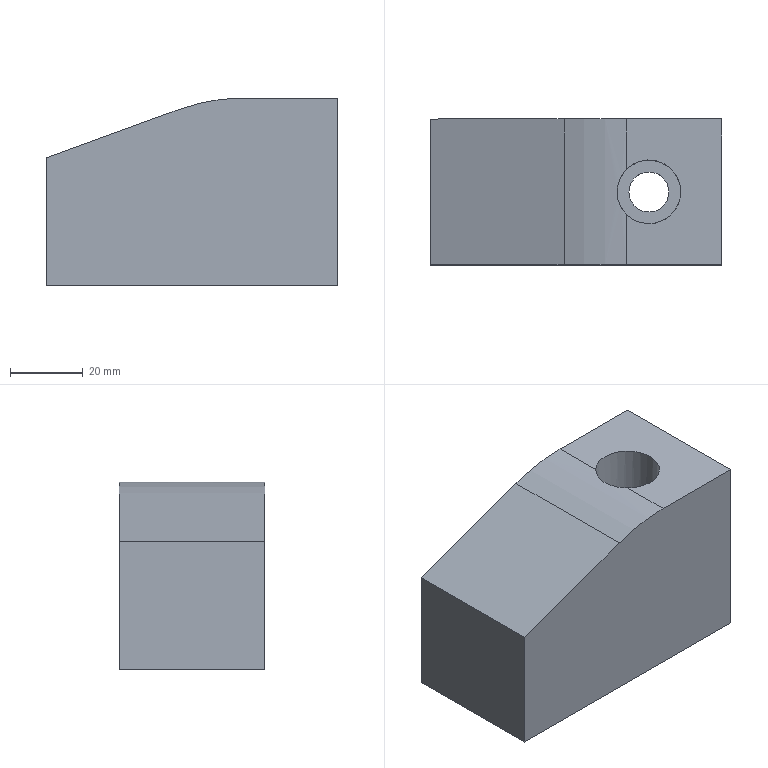Part | NX | features MAIN_BODY 2 | 1 solid | 11 faces | box 80 x 40 x 51.5 mm | volume 139981 mm3 | plane 8 | cylinder 3 | commonest cylinder face diameters 11 x1 17.5 x1 100 x1
STEP:
#1=CARTESIAN_POINT('',(-1566.191,130.,-4.));
#2=VERTEX_POINT('',#1);
#3=CARTESIAN_POINT('',(-1540.,130.,-4.));
#4=VERTEX_POINT('',#3);
#5=CARTESIAN_POINT('',(-1625.,130.,-4.));
#6=DIRECTION('',(-1.,0.,0.));
#7=VECTOR('',#6,1000.);
#8=LINE('',#5,#7);
#9=EDGE_CURVE('',#2,#4,#8,.F.);
#10=ORIENTED_EDGE('',*,*,#9,.F.);
#11=CARTESIAN_POINT('',(-1583.278,130.,-7.01));
#12=VERTEX_POINT('',#11);
#13=CARTESIAN_POINT('',(-1566.191,130.,-54.));
#14=DIRECTION('',(0.,1.,0.));
#15=DIRECTION('',(0.,0.,1.));
#16=AXIS2_PLACEMENT_3D('',#13,#14,#15);
#17=CIRCLE('',#16,50.);
#18=EDGE_CURVE('',#2,#12,#17,.F.);
#19=ORIENTED_EDGE('',*,*,#18,.T.);
#20=CARTESIAN_POINT('',(-1620.,130.,-20.364));
#21=VERTEX_POINT('',#20);
#22=CARTESIAN_POINT('',(-1619.161,130.,-20.058));
#23=DIRECTION('',(-0.9398,0.,-0.3417));
#24=VECTOR('',#23,1000.);
#25=LINE('',#22,#24);
#26=EDGE_CURVE('',#12,#21,#25,.T.);
#27=ORIENTED_EDGE('',*,*,#26,.T.);
#28=CARTESIAN_POINT('',(-1620.,130.,-55.5));
#29=VERTEX_POINT('',#28);
#30=CARTESIAN_POINT('',(-1620.,130.,-4.));
#31=DIRECTION('',(0.,0.,1.));
#32=VECTOR('',#31,1000.);
#33=LINE('',#30,#32);
#34=EDGE_CURVE('',#21,#29,#33,.F.);
#35=ORIENTED_EDGE('',*,*,#34,.T.);
#36=CARTESIAN_POINT('',(-1540.,130.,-55.5));
#37=VERTEX_POINT('',#36);
#38=CARTESIAN_POINT('',(-1625.,130.,-55.5));
#39=DIRECTION('',(-1.,0.,0.));
#40=VECTOR('',#39,1000.);
#41=LINE('',#38,#40);
#42=EDGE_CURVE('',#29,#37,#41,.F.);
#43=ORIENTED_EDGE('',*,*,#42,.T.);
#44=CARTESIAN_POINT('',(-1540.,130.,-4.));
#45=DIRECTION('',(0.,0.,1.));
#46=VECTOR('',#45,1000.);
#47=LINE('',#44,#46);
#48=EDGE_CURVE('',#4,#37,#47,.F.);
#49=ORIENTED_EDGE('',*,*,#48,.F.);
#50=EDGE_LOOP('',(#10,#19,#27,#35,#43,#49));
#51=FACE_BOUND('',#50,.T.);
#52=CARTESIAN_POINT('',(-1625.,130.,-4.));
#53=DIRECTION('',(0.,1.,0.));
#54=DIRECTION('',(0.,0.,-1.));
#55=AXIS2_PLACEMENT_3D('',#52,#53,#54);
#56=PLANE('',#55);
#57=ADVANCED_FACE('',(#51),#56,.F.);
#58=CARTESIAN_POINT('',(-1620.,170.,-20.364));
#59=VERTEX_POINT('',#58);
#60=CARTESIAN_POINT('',(-1583.278,170.,-7.01));
#61=VERTEX_POINT('',#60);
#62=CARTESIAN_POINT('',(-1619.161,170.,-20.058));
#63=DIRECTION('',(-0.9398,0.,-0.3417));
#64=VECTOR('',#63,1000.);
#65=LINE('',#62,#64);
#66=EDGE_CURVE('',#59,#61,#65,.F.);
#67=ORIENTED_EDGE('',*,*,#66,.T.);
#68=CARTESIAN_POINT('',(-1566.191,170.,-4.));
#69=VERTEX_POINT('',#68);
#70=CARTESIAN_POINT('',(-1566.191,170.,-54.));
#71=DIRECTION('',(0.,1.,0.));
#72=DIRECTION('',(0.,0.,1.));
#73=AXIS2_PLACEMENT_3D('',#70,#71,#72);
#74=CIRCLE('',#73,50.);
#75=EDGE_CURVE('',#61,#69,#74,.T.);
#76=ORIENTED_EDGE('',*,*,#75,.T.);
#77=CARTESIAN_POINT('',(-1540.,170.,-4.));
#78=VERTEX_POINT('',#77);
#79=CARTESIAN_POINT('',(-1625.,170.,-4.));
#80=DIRECTION('',(1.,0.,0.));
#81=VECTOR('',#80,1000.);
#82=LINE('',#79,#81);
#83=EDGE_CURVE('',#69,#78,#82,.T.);
#84=ORIENTED_EDGE('',*,*,#83,.T.);
#85=CARTESIAN_POINT('',(-1540.,170.,-55.5));
#86=VERTEX_POINT('',#85);
#87=CARTESIAN_POINT('',(-1540.,170.,-4.));
#88=DIRECTION('',(0.,0.,-1.));
#89=VECTOR('',#88,1000.);
#90=LINE('',#87,#89);
#91=EDGE_CURVE('',#78,#86,#90,.T.);
#92=ORIENTED_EDGE('',*,*,#91,.T.);
#93=CARTESIAN_POINT('',(-1620.,170.,-55.5));
#94=VERTEX_POINT('',#93);
#95=CARTESIAN_POINT('',(-1625.,170.,-55.5));
#96=DIRECTION('',(-1.,0.,0.));
#97=VECTOR('',#96,1000.);
#98=LINE('',#95,#97);
#99=EDGE_CURVE('',#86,#94,#98,.T.);
#100=ORIENTED_EDGE('',*,*,#99,.T.);
#101=CARTESIAN_POINT('',(-1620.,170.,-4.));
#102=DIRECTION('',(0.,0.,-1.));
#103=VECTOR('',#102,1000.);
#104=LINE('',#101,#103);
#105=EDGE_CURVE('',#59,#94,#104,.T.);
#106=ORIENTED_EDGE('',*,*,#105,.F.);
#107=EDGE_LOOP('',(#67,#76,#84,#92,#100,#106));
#108=FACE_BOUND('',#107,.T.);
#109=CARTESIAN_POINT('',(-1625.,170.,-4.));
#110=DIRECTION('',(0.,1.,0.));
#111=DIRECTION('',(0.,0.,-1.));
#112=AXIS2_PLACEMENT_3D('',#109,#110,#111);
#113=PLANE('',#112);
#114=ADVANCED_FACE('',(#108),#113,.T.);
#115=ORIENTED_EDGE('',*,*,#48,.T.);
#116=CARTESIAN_POINT('',(-1540.,135.,-55.5));
#117=DIRECTION('',(0.,-1.,0.));
#118=VECTOR('',#117,1000.);
#119=LINE('',#116,#118);
#120=EDGE_CURVE('',#86,#37,#119,.T.);
#121=ORIENTED_EDGE('',*,*,#120,.F.);
#122=ORIENTED_EDGE('',*,*,#91,.F.);
#123=CARTESIAN_POINT('',(-1540.,135.,-4.));
#124=DIRECTION('',(0.,1.,0.));
#125=VECTOR('',#124,1000.);
#126=LINE('',#123,#125);
#127=EDGE_CURVE('',#4,#78,#126,.T.);
#128=ORIENTED_EDGE('',*,*,#127,.F.);
#129=EDGE_LOOP('',(#115,#121,#122,#128));
#130=FACE_BOUND('',#129,.T.);
#131=CARTESIAN_POINT('',(-1540.,135.,-4.));
#132=DIRECTION('',(-1.,0.,0.));
#133=DIRECTION('',(0.,0.,1.));
#134=AXIS2_PLACEMENT_3D('',#131,#132,#133);
#135=PLANE('',#134);
#136=ADVANCED_FACE('',(#130),#135,.F.);
#137=ORIENTED_EDGE('',*,*,#105,.T.);
#138=CARTESIAN_POINT('',(-1620.,135.,-55.5));
#139=DIRECTION('',(0.,-1.,0.));
#140=VECTOR('',#139,1000.);
#141=LINE('',#138,#140);
#142=EDGE_CURVE('',#94,#29,#141,.T.);
#143=ORIENTED_EDGE('',*,*,#142,.T.);
#144=ORIENTED_EDGE('',*,*,#34,.F.);
#145=CARTESIAN_POINT('',(-1620.,135.,-20.364));
#146=DIRECTION('',(0.,-1.,0.));
#147=VECTOR('',#146,1000.);
#148=LINE('',#145,#147);
#149=EDGE_CURVE('',#21,#59,#148,.F.);
#150=ORIENTED_EDGE('',*,*,#149,.T.);
#151=EDGE_LOOP('',(#137,#143,#144,#150));
#152=FACE_BOUND('',#151,.T.);
#153=CARTESIAN_POINT('',(-1620.,135.,-4.));
#154=DIRECTION('',(-1.,0.,0.));
#155=DIRECTION('',(0.,0.,1.));
#156=AXIS2_PLACEMENT_3D('',#153,#154,#155);
#157=PLANE('',#156);
#158=ADVANCED_FACE('',(#152),#157,.T.);
#159=CARTESIAN_POINT('',(-1566.191,156.183,-4.));
#160=VERTEX_POINT('',#159);
#161=CARTESIAN_POINT('',(-1566.191,135.,-4.));
#162=DIRECTION('',(0.,1.,0.));
#163=VECTOR('',#162,1000.);
#164=LINE('',#161,#163);
#165=EDGE_CURVE('',#69,#160,#164,.F.);
#166=ORIENTED_EDGE('',*,*,#165,.T.);
#167=CARTESIAN_POINT('',(-1566.191,143.817,-4.));
#168=VERTEX_POINT('',#167);
#169=CARTESIAN_POINT('',(-1560.,150.,-4.));
#170=DIRECTION('',(0.,0.,-1.));
#171=DIRECTION('',(1.,0.,0.));
#172=AXIS2_PLACEMENT_3D('',#169,#170,#171);
#173=CIRCLE('',#172,8.75);
#174=EDGE_CURVE('',#168,#160,#173,.F.);
#175=ORIENTED_EDGE('',*,*,#174,.F.);
#176=CARTESIAN_POINT('',(-1566.191,135.,-4.));
#177=DIRECTION('',(0.,1.,0.));
#178=VECTOR('',#177,1000.);
#179=LINE('',#176,#178);
#180=EDGE_CURVE('',#168,#2,#179,.F.);
#181=ORIENTED_EDGE('',*,*,#180,.T.);
#182=ORIENTED_EDGE('',*,*,#9,.T.);
#183=ORIENTED_EDGE('',*,*,#127,.T.);
#184=ORIENTED_EDGE('',*,*,#83,.F.);
#185=EDGE_LOOP('',(#166,#175,#181,#182,#183,#184));
#186=FACE_BOUND('',#185,.T.);
#187=CARTESIAN_POINT('',(-1625.,135.,-4.));
#188=DIRECTION('',(0.,0.,1.));
#189=DIRECTION('',(0.,1.,0.));
#190=AXIS2_PLACEMENT_3D('',#187,#188,#189);
#191=PLANE('',#190);
#192=ADVANCED_FACE('',(#186),#191,.T.);
#193=ORIENTED_EDGE('',*,*,#26,.F.);
#194=CARTESIAN_POINT('',(-1583.278,135.,-7.01));
#195=DIRECTION('',(0.,-1.,0.));
#196=VECTOR('',#195,1000.);
#197=LINE('',#194,#196);
#198=EDGE_CURVE('',#12,#61,#197,.F.);
#199=ORIENTED_EDGE('',*,*,#198,.T.);
#200=ORIENTED_EDGE('',*,*,#66,.F.);
#201=ORIENTED_EDGE('',*,*,#149,.F.);
#202=EDGE_LOOP('',(#193,#199,#200,#201));
#203=FACE_BOUND('',#202,.T.);
#204=CARTESIAN_POINT('',(-1630.,135.,-24.));
#205=DIRECTION('',(0.3417,0.,-0.9398));
#206=DIRECTION('',(-0.9398,0.,-0.3417));
#207=AXIS2_PLACEMENT_3D('',#204,#205,#206);
#208=PLANE('',#207);
#209=ADVANCED_FACE('',(#203),#208,.F.);
#210=ORIENTED_EDGE('',*,*,#180,.F.);
#211=CARTESIAN_POINT('',(-1566.191,156.183,-4.));
#212=CARTESIAN_POINT('',(-1567.825,154.548,-4.));
#213=CARTESIAN_POINT('',(-1569.686,150.004,-4.131));
#214=CARTESIAN_POINT('',(-1567.803,145.431,-4.));
#215=CARTESIAN_POINT('',(-1566.191,143.817,-4.));
#216=B_SPLINE_CURVE_WITH_KNOTS('',3,(#211,#212,#213,#214,#215),.UNSPECIFIED.,.F.,.F.,(4,1,4),(0.002912,0.009748,0.01658),.UNSPECIFIED.);
#217=EDGE_CURVE('',#168,#160,#216,.F.);
#218=ORIENTED_EDGE('',*,*,#217,.T.);
#219=ORIENTED_EDGE('',*,*,#165,.F.);
#220=ORIENTED_EDGE('',*,*,#75,.F.);
#221=ORIENTED_EDGE('',*,*,#198,.F.);
#222=ORIENTED_EDGE('',*,*,#18,.F.);
#223=EDGE_LOOP('',(#210,#218,#219,#220,#221,#222));
#224=FACE_BOUND('',#223,.T.);
#225=CARTESIAN_POINT('',(-1566.191,135.,-54.));
#226=DIRECTION('',(0.,1.,0.));
#227=DIRECTION('',(0.,0.,1.));
#228=AXIS2_PLACEMENT_3D('',#225,#226,#227);
#229=CYLINDRICAL_SURFACE('',#228,50.);
#230=ADVANCED_FACE('',(#224),#229,.T.);
#231=CARTESIAN_POINT('',(-1565.5,150.,-38.5));
#232=VERTEX_POINT('',#231);
#233=CARTESIAN_POINT('',(-1560.,150.,-38.5));
#234=DIRECTION('',(0.,0.,-1.));
#235=DIRECTION('',(-1.,0.,0.));
#236=AXIS2_PLACEMENT_3D('',#233,#234,#235);
#237=CIRCLE('',#236,5.5);
#238=EDGE_CURVE('',#232,#232,#237,.T.);
#239=ORIENTED_EDGE('',*,*,#238,.F.);
#240=EDGE_LOOP('',(#239));
#241=FACE_BOUND('',#240,.T.);
#242=CARTESIAN_POINT('',(-1565.5,150.,-55.5));
#243=VERTEX_POINT('',#242);
#244=CARTESIAN_POINT('',(-1560.,150.,-55.5));
#245=DIRECTION('',(0.,0.,-1.));
#246=DIRECTION('',(-1.,0.,0.));
#247=AXIS2_PLACEMENT_3D('',#244,#245,#246);
#248=CIRCLE('',#247,5.5);
#249=EDGE_CURVE('',#243,#243,#248,.T.);
#250=ORIENTED_EDGE('',*,*,#249,.T.);
#251=EDGE_LOOP('',(#250));
#252=FACE_BOUND('',#251,.T.);
#253=CARTESIAN_POINT('',(-1560.,150.,-54.));
#254=DIRECTION('',(0.,0.,-1.));
#255=DIRECTION('',(-1.,0.,0.));
#256=AXIS2_PLACEMENT_3D('',#253,#254,#255);
#257=CYLINDRICAL_SURFACE('',#256,5.5);
#258=ADVANCED_FACE('',(#241,#252),#257,.F.);
#259=ORIENTED_EDGE('',*,*,#238,.T.);
#260=EDGE_LOOP('',(#259));
#261=FACE_BOUND('',#260,.T.);
#262=CARTESIAN_POINT('',(-1568.75,150.,-38.5));
#263=VERTEX_POINT('',#262);
#264=CARTESIAN_POINT('',(-1560.,150.,-38.5));
#265=DIRECTION('',(0.,0.,-1.));
#266=DIRECTION('',(-1.,0.,0.));
#267=AXIS2_PLACEMENT_3D('',#264,#265,#266);
#268=CIRCLE('',#267,8.75);
#269=EDGE_CURVE('',#263,#263,#268,.T.);
#270=ORIENTED_EDGE('',*,*,#269,.F.);
#271=EDGE_LOOP('',(#270));
#272=FACE_BOUND('',#271,.T.);
#273=CARTESIAN_POINT('',(-1585.,150.,-38.5));
#274=DIRECTION('',(0.,0.,-1.));
#275=DIRECTION('',(-1.,0.,0.));
#276=AXIS2_PLACEMENT_3D('',#273,#274,#275);
#277=PLANE('',#276);
#278=ADVANCED_FACE('',(#261,#272),#277,.F.);
#279=ORIENTED_EDGE('',*,*,#217,.F.);
#280=ORIENTED_EDGE('',*,*,#174,.T.);
#281=EDGE_LOOP('',(#279,#280));
#282=FACE_BOUND('',#281,.T.);
#283=ORIENTED_EDGE('',*,*,#269,.T.);
#284=EDGE_LOOP('',(#283));
#285=FACE_BOUND('',#284,.T.);
#286=CARTESIAN_POINT('',(-1560.,150.,-4.));
#287=DIRECTION('',(0.,0.,-1.));
#288=DIRECTION('',(-1.,0.,0.));
#289=AXIS2_PLACEMENT_3D('',#286,#287,#288);
#290=CYLINDRICAL_SURFACE('',#289,8.75);
#291=ADVANCED_FACE('',(#282,#285),#290,.F.);
#292=ORIENTED_EDGE('',*,*,#249,.F.);
#293=EDGE_LOOP('',(#292));
#294=FACE_BOUND('',#293,.T.);
#295=ORIENTED_EDGE('',*,*,#99,.F.);
#296=ORIENTED_EDGE('',*,*,#120,.T.);
#297=ORIENTED_EDGE('',*,*,#42,.F.);
#298=ORIENTED_EDGE('',*,*,#142,.F.);
#299=EDGE_LOOP('',(#295,#296,#297,#298));
#300=FACE_BOUND('',#299,.T.);
#301=CARTESIAN_POINT('',(-1590.,155.,-55.5));
#302=DIRECTION('',(0.,0.,-1.));
#303=DIRECTION('',(-1.,0.,0.));
#304=AXIS2_PLACEMENT_3D('',#301,#302,#303);
#305=PLANE('',#304);
#306=ADVANCED_FACE('',(#294,#300),#305,.T.);
#307=CLOSED_SHELL('',(#57,#114,#136,#158,#192,#209,#230,#258,#278,#291,#306));
#308=MANIFOLD_SOLID_BREP('',#307);
#309=(LENGTH_UNIT()NAMED_UNIT(*)SI_UNIT(.MILLI.,.METRE.));
#310=UNCERTAINTY_MEASURE_WITH_UNIT(LENGTH_MEASURE(0.0508),#309,'','');
#311=(NAMED_UNIT(*)PLANE_ANGLE_UNIT()SI_UNIT($,.RADIAN.));
#312=(NAMED_UNIT(*)SI_UNIT($,.STERADIAN.)SOLID_ANGLE_UNIT());
#313=(GEOMETRIC_REPRESENTATION_CONTEXT(3)GLOBAL_UNCERTAINTY_ASSIGNED_CONTEXT((#310))GLOBAL_UNIT_ASSIGNED_CONTEXT((#309,#311,#312))REPRESENTATION_CONTEXT('',''));
#314=ADVANCED_BREP_SHAPE_REPRESENTATION('',(#308),#313);